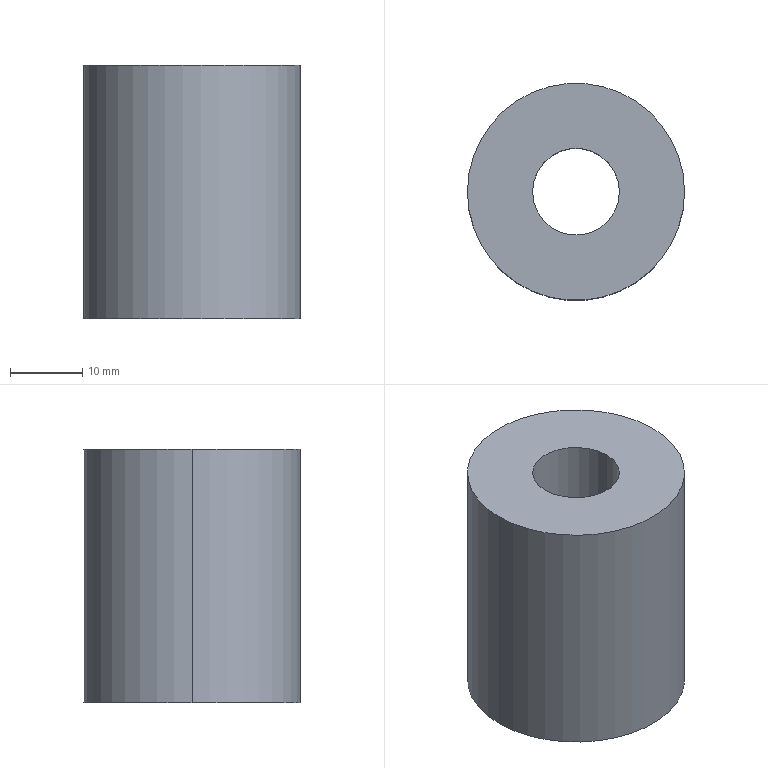Part | SolidWorks | features ICE 2, Extrusion 1 | 1 solid | 9 faces | box 30 x 30 x 35 mm | volume 19242 mm3 | cylinder 6 | plane 3 | commonest cylinder face diameters 12 x2 16 x2 30 x2
STEP:
#1=CARTESIAN_POINT('',(8.,0.,17.5));
#2=VERTEX_POINT('',#1);
#3=CARTESIAN_POINT('',(-8.,0.,17.5));
#4=VERTEX_POINT('',#3);
#5=CARTESIAN_POINT('',(0.,0.,17.5));
#6=DIRECTION('',(0.,0.,-1.));
#7=DIRECTION('',(-1.,0.,0.));
#8=AXIS2_PLACEMENT_3D('',#5,#6,#7);
#9=CIRCLE('',#8,8.);
#10=EDGE_CURVE('',#2,#4,#9,.T.);
#11=ORIENTED_EDGE('',*,*,#10,.F.);
#12=CARTESIAN_POINT('',(8.,0.,0.));
#13=VERTEX_POINT('',#12);
#14=CARTESIAN_POINT('',(8.,0.,17.5));
#15=DIRECTION('',(0.,0.,-1.));
#16=VECTOR('',#15,1000.);
#17=LINE('',#14,#16);
#18=EDGE_CURVE('',#2,#13,#17,.T.);
#19=ORIENTED_EDGE('',*,*,#18,.T.);
#20=CARTESIAN_POINT('',(-8.,0.,0.));
#21=VERTEX_POINT('',#20);
#22=CARTESIAN_POINT('',(0.,0.,0.));
#23=DIRECTION('',(0.,0.,-1.));
#24=DIRECTION('',(-1.,0.,0.));
#25=AXIS2_PLACEMENT_3D('',#22,#23,#24);
#26=CIRCLE('',#25,8.);
#27=EDGE_CURVE('',#13,#21,#26,.T.);
#28=ORIENTED_EDGE('',*,*,#27,.T.);
#29=CARTESIAN_POINT('',(-8.,0.,17.5));
#30=DIRECTION('',(0.,0.,-1.));
#31=VECTOR('',#30,1000.);
#32=LINE('',#29,#31);
#33=EDGE_CURVE('',#4,#21,#32,.T.);
#34=ORIENTED_EDGE('',*,*,#33,.F.);
#35=EDGE_LOOP('',(#11,#19,#28,#34));
#36=FACE_OUTER_BOUND('',#35,.T.);
#37=CARTESIAN_POINT('',(0.,0.,17.5));
#38=DIRECTION('',(0.,0.,-1.));
#39=DIRECTION('',(-1.,0.,0.));
#40=AXIS2_PLACEMENT_3D('',#37,#38,#39);
#41=CYLINDRICAL_SURFACE('',#40,8.);
#42=ADVANCED_FACE('',(#36),#41,.F.);
#43=CARTESIAN_POINT('',(-6.,0.,17.5));
#44=VERTEX_POINT('',#43);
#45=CARTESIAN_POINT('',(6.,0.,17.5));
#46=VERTEX_POINT('',#45);
#47=CARTESIAN_POINT('',(0.,0.,17.5));
#48=DIRECTION('',(0.,0.,1.));
#49=DIRECTION('',(-1.,0.,0.));
#50=AXIS2_PLACEMENT_3D('',#47,#48,#49);
#51=CIRCLE('',#50,6.);
#52=EDGE_CURVE('',#44,#46,#51,.T.);
#53=ORIENTED_EDGE('',*,*,#52,.F.);
#54=CARTESIAN_POINT('',(-6.,0.,35.));
#55=VERTEX_POINT('',#54);
#56=CARTESIAN_POINT('',(-6.,0.,17.5));
#57=DIRECTION('',(0.,0.,1.));
#58=VECTOR('',#57,1000.);
#59=LINE('',#56,#58);
#60=EDGE_CURVE('',#44,#55,#59,.T.);
#61=ORIENTED_EDGE('',*,*,#60,.T.);
#62=CARTESIAN_POINT('',(6.,0.,35.));
#63=VERTEX_POINT('',#62);
#64=CARTESIAN_POINT('',(0.,0.,35.));
#65=DIRECTION('',(0.,0.,1.));
#66=DIRECTION('',(1.,0.,0.));
#67=AXIS2_PLACEMENT_3D('',#64,#65,#66);
#68=CIRCLE('',#67,6.);
#69=EDGE_CURVE('',#55,#63,#68,.T.);
#70=ORIENTED_EDGE('',*,*,#69,.T.);
#71=CARTESIAN_POINT('',(6.,0.,17.5));
#72=DIRECTION('',(0.,0.,1.));
#73=VECTOR('',#72,1000.);
#74=LINE('',#71,#73);
#75=EDGE_CURVE('',#46,#63,#74,.T.);
#76=ORIENTED_EDGE('',*,*,#75,.F.);
#77=EDGE_LOOP('',(#53,#61,#70,#76));
#78=FACE_OUTER_BOUND('',#77,.T.);
#79=CARTESIAN_POINT('',(0.,0.,17.5));
#80=DIRECTION('',(0.,0.,1.));
#81=DIRECTION('',(1.,0.,0.));
#82=AXIS2_PLACEMENT_3D('',#79,#80,#81);
#83=CYLINDRICAL_SURFACE('',#82,6.);
#84=ADVANCED_FACE('',(#78),#83,.F.);
#85=CARTESIAN_POINT('',(15.,0.,35.));
#86=VERTEX_POINT('',#85);
#87=CARTESIAN_POINT('',(-15.,0.,35.));
#88=VERTEX_POINT('',#87);
#89=CARTESIAN_POINT('',(0.,0.,35.));
#90=DIRECTION('',(0.,0.,1.));
#91=DIRECTION('',(1.,0.,0.));
#92=AXIS2_PLACEMENT_3D('',#89,#90,#91);
#93=CIRCLE('',#92,15.);
#94=EDGE_CURVE('',#86,#88,#93,.T.);
#95=ORIENTED_EDGE('',*,*,#94,.F.);
#96=CARTESIAN_POINT('',(15.,0.,0.));
#97=VERTEX_POINT('',#96);
#98=CARTESIAN_POINT('',(15.,0.,35.));
#99=DIRECTION('',(0.,0.,-1.));
#100=VECTOR('',#99,1000.);
#101=LINE('',#98,#100);
#102=EDGE_CURVE('',#86,#97,#101,.T.);
#103=ORIENTED_EDGE('',*,*,#102,.T.);
#104=CARTESIAN_POINT('',(-15.,0.,0.));
#105=VERTEX_POINT('',#104);
#106=CARTESIAN_POINT('',(0.,0.,0.));
#107=DIRECTION('',(0.,0.,1.));
#108=DIRECTION('',(1.,0.,0.));
#109=AXIS2_PLACEMENT_3D('',#106,#107,#108);
#110=CIRCLE('',#109,15.);
#111=EDGE_CURVE('',#97,#105,#110,.T.);
#112=ORIENTED_EDGE('',*,*,#111,.T.);
#113=CARTESIAN_POINT('',(-15.,0.,35.));
#114=DIRECTION('',(0.,0.,-1.));
#115=VECTOR('',#114,1000.);
#116=LINE('',#113,#115);
#117=EDGE_CURVE('',#88,#105,#116,.T.);
#118=ORIENTED_EDGE('',*,*,#117,.F.);
#119=EDGE_LOOP('',(#95,#103,#112,#118));
#120=FACE_OUTER_BOUND('',#119,.T.);
#121=CARTESIAN_POINT('',(0.,0.,35.));
#122=DIRECTION('',(0.,0.,-1.));
#123=DIRECTION('',(-1.,0.,0.));
#124=AXIS2_PLACEMENT_3D('',#121,#122,#123);
#125=CYLINDRICAL_SURFACE('',#124,15.);
#126=ADVANCED_FACE('',(#120),#125,.T.);
#127=ORIENTED_EDGE('',*,*,#102,.F.);
#128=CARTESIAN_POINT('',(0.,0.,35.));
#129=DIRECTION('',(0.,0.,1.));
#130=DIRECTION('',(1.,0.,0.));
#131=AXIS2_PLACEMENT_3D('',#128,#129,#130);
#132=CIRCLE('',#131,15.);
#133=EDGE_CURVE('',#88,#86,#132,.T.);
#134=ORIENTED_EDGE('',*,*,#133,.F.);
#135=ORIENTED_EDGE('',*,*,#117,.T.);
#136=CARTESIAN_POINT('',(0.,0.,0.));
#137=DIRECTION('',(0.,0.,1.));
#138=DIRECTION('',(1.,0.,0.));
#139=AXIS2_PLACEMENT_3D('',#136,#137,#138);
#140=CIRCLE('',#139,15.);
#141=EDGE_CURVE('',#105,#97,#140,.T.);
#142=ORIENTED_EDGE('',*,*,#141,.T.);
#143=EDGE_LOOP('',(#127,#134,#135,#142));
#144=FACE_OUTER_BOUND('',#143,.T.);
#145=CARTESIAN_POINT('',(0.,0.,35.));
#146=DIRECTION('',(0.,0.,-1.));
#147=DIRECTION('',(-1.,0.,0.));
#148=AXIS2_PLACEMENT_3D('',#145,#146,#147);
#149=CYLINDRICAL_SURFACE('',#148,15.);
#150=ADVANCED_FACE('',(#144),#149,.T.);
#151=CARTESIAN_POINT('',(0.,0.,35.));
#152=DIRECTION('',(0.,0.,1.));
#153=DIRECTION('',(1.,0.,0.));
#154=AXIS2_PLACEMENT_3D('',#151,#152,#153);
#155=CIRCLE('',#154,6.);
#156=EDGE_CURVE('',#63,#55,#155,.T.);
#157=ORIENTED_EDGE('',*,*,#156,.F.);
#158=ORIENTED_EDGE('',*,*,#69,.F.);
#159=EDGE_LOOP('',(#157,#158));
#160=FACE_BOUND('',#159,.T.);
#161=ORIENTED_EDGE('',*,*,#133,.T.);
#162=ORIENTED_EDGE('',*,*,#94,.T.);
#163=EDGE_LOOP('',(#161,#162));
#164=FACE_OUTER_BOUND('',#163,.T.);
#165=CARTESIAN_POINT('',(0.,0.,35.));
#166=DIRECTION('',(0.,0.,1.));
#167=DIRECTION('',(1.,0.,0.));
#168=AXIS2_PLACEMENT_3D('',#165,#166,#167);
#169=PLANE('',#168);
#170=ADVANCED_FACE('',(#160,#164),#169,.T.);
#171=CARTESIAN_POINT('',(0.,0.,0.));
#172=DIRECTION('',(0.,0.,-1.));
#173=DIRECTION('',(-1.,0.,0.));
#174=AXIS2_PLACEMENT_3D('',#171,#172,#173);
#175=CIRCLE('',#174,8.);
#176=EDGE_CURVE('',#21,#13,#175,.T.);
#177=ORIENTED_EDGE('',*,*,#176,.F.);
#178=ORIENTED_EDGE('',*,*,#27,.F.);
#179=EDGE_LOOP('',(#177,#178));
#180=FACE_BOUND('',#179,.T.);
#181=ORIENTED_EDGE('',*,*,#141,.F.);
#182=ORIENTED_EDGE('',*,*,#111,.F.);
#183=EDGE_LOOP('',(#181,#182));
#184=FACE_OUTER_BOUND('',#183,.T.);
#185=CARTESIAN_POINT('',(0.,0.,0.));
#186=DIRECTION('',(0.,0.,1.));
#187=DIRECTION('',(1.,0.,0.));
#188=AXIS2_PLACEMENT_3D('',#185,#186,#187);
#189=PLANE('',#188);
#190=ADVANCED_FACE('',(#180,#184),#189,.F.);
#191=ORIENTED_EDGE('',*,*,#60,.F.);
#192=CARTESIAN_POINT('',(0.,0.,17.5));
#193=DIRECTION('',(0.,0.,1.));
#194=DIRECTION('',(-1.,0.,0.));
#195=AXIS2_PLACEMENT_3D('',#192,#193,#194);
#196=CIRCLE('',#195,6.);
#197=EDGE_CURVE('',#46,#44,#196,.T.);
#198=ORIENTED_EDGE('',*,*,#197,.F.);
#199=ORIENTED_EDGE('',*,*,#75,.T.);
#200=ORIENTED_EDGE('',*,*,#156,.T.);
#201=EDGE_LOOP('',(#191,#198,#199,#200));
#202=FACE_OUTER_BOUND('',#201,.T.);
#203=CARTESIAN_POINT('',(0.,0.,17.5));
#204=DIRECTION('',(0.,0.,1.));
#205=DIRECTION('',(1.,0.,0.));
#206=AXIS2_PLACEMENT_3D('',#203,#204,#205);
#207=CYLINDRICAL_SURFACE('',#206,6.);
#208=ADVANCED_FACE('',(#202),#207,.F.);
#209=CARTESIAN_POINT('',(0.,0.,17.5));
#210=DIRECTION('',(0.,0.,-1.));
#211=DIRECTION('',(-1.,0.,0.));
#212=AXIS2_PLACEMENT_3D('',#209,#210,#211);
#213=CIRCLE('',#212,8.);
#214=EDGE_CURVE('',#4,#2,#213,.T.);
#215=ORIENTED_EDGE('',*,*,#214,.T.);
#216=ORIENTED_EDGE('',*,*,#10,.T.);
#217=EDGE_LOOP('',(#215,#216));
#218=FACE_OUTER_BOUND('',#217,.T.);
#219=ORIENTED_EDGE('',*,*,#197,.T.);
#220=ORIENTED_EDGE('',*,*,#52,.T.);
#221=EDGE_LOOP('',(#219,#220));
#222=FACE_BOUND('',#221,.T.);
#223=CARTESIAN_POINT('',(0.,0.,17.5));
#224=DIRECTION('',(0.,0.,-1.));
#225=DIRECTION('',(-1.,0.,0.));
#226=AXIS2_PLACEMENT_3D('',#223,#224,#225);
#227=PLANE('',#226);
#228=ADVANCED_FACE('',(#218,#222),#227,.T.);
#229=ORIENTED_EDGE('',*,*,#18,.F.);
#230=ORIENTED_EDGE('',*,*,#214,.F.);
#231=ORIENTED_EDGE('',*,*,#33,.T.);
#232=ORIENTED_EDGE('',*,*,#176,.T.);
#233=EDGE_LOOP('',(#229,#230,#231,#232));
#234=FACE_OUTER_BOUND('',#233,.T.);
#235=CARTESIAN_POINT('',(0.,0.,17.5));
#236=DIRECTION('',(0.,0.,-1.));
#237=DIRECTION('',(-1.,0.,0.));
#238=AXIS2_PLACEMENT_3D('',#235,#236,#237);
#239=CYLINDRICAL_SURFACE('',#238,8.);
#240=ADVANCED_FACE('',(#234),#239,.F.);
#241=CLOSED_SHELL('',(#42,#84,#126,#150,#170,#190,#208,#228,#240));
#242=MANIFOLD_SOLID_BREP('',#241);
#243=CARTESIAN_POINT('',(0.,0.,0.));
#244=DIRECTION('',(0.,0.,1.));
#245=DIRECTION('',(1.,0.,0.));
#246=AXIS2_PLACEMENT_3D('',#243,#244,#245);
#247=(LENGTH_UNIT()NAMED_UNIT(*)SI_UNIT(.MILLI.,.METRE.));
#248=UNCERTAINTY_MEASURE_WITH_UNIT(LENGTH_MEASURE(0.00001),#247,'','');
#249=(NAMED_UNIT(*)PLANE_ANGLE_UNIT()SI_UNIT($,.RADIAN.));
#250=(NAMED_UNIT(*)SI_UNIT($,.STERADIAN.)SOLID_ANGLE_UNIT());
#251=(GEOMETRIC_REPRESENTATION_CONTEXT(3)GLOBAL_UNCERTAINTY_ASSIGNED_CONTEXT((#248))GLOBAL_UNIT_ASSIGNED_CONTEXT((#247,#249,#250))REPRESENTATION_CONTEXT('',''));
#252=ADVANCED_BREP_SHAPE_REPRESENTATION('',(#242,#246),#251);